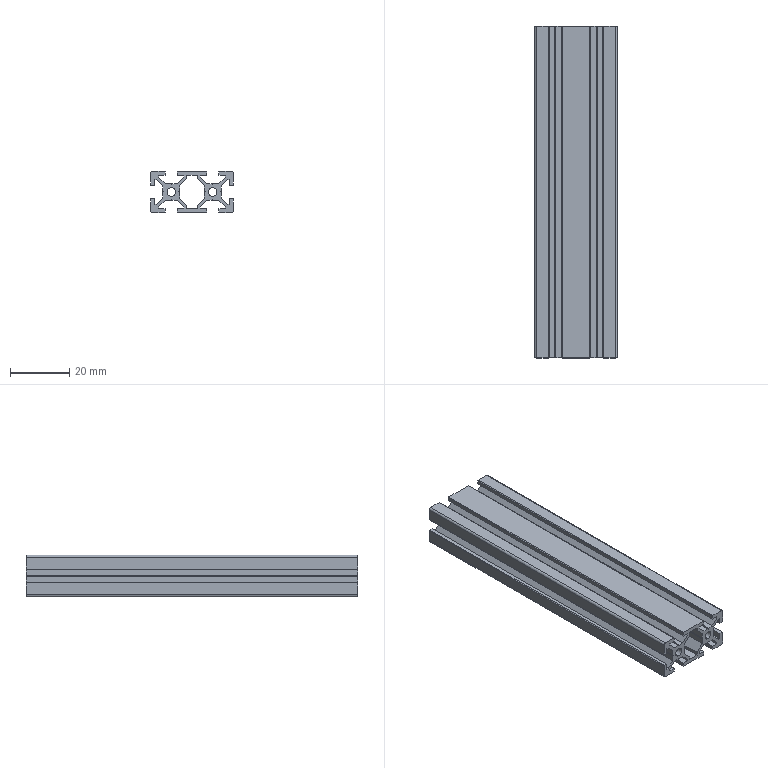Part | SolidWorks | features SplitBody 1 | 1 solid | 122 faces | box 28 x 112 x 14 mm | volume 17760 mm3 | plane 102 | cylinder 20 | commonest cylinder face diameters 0.42 x12 1.4 x4 2.8 x4